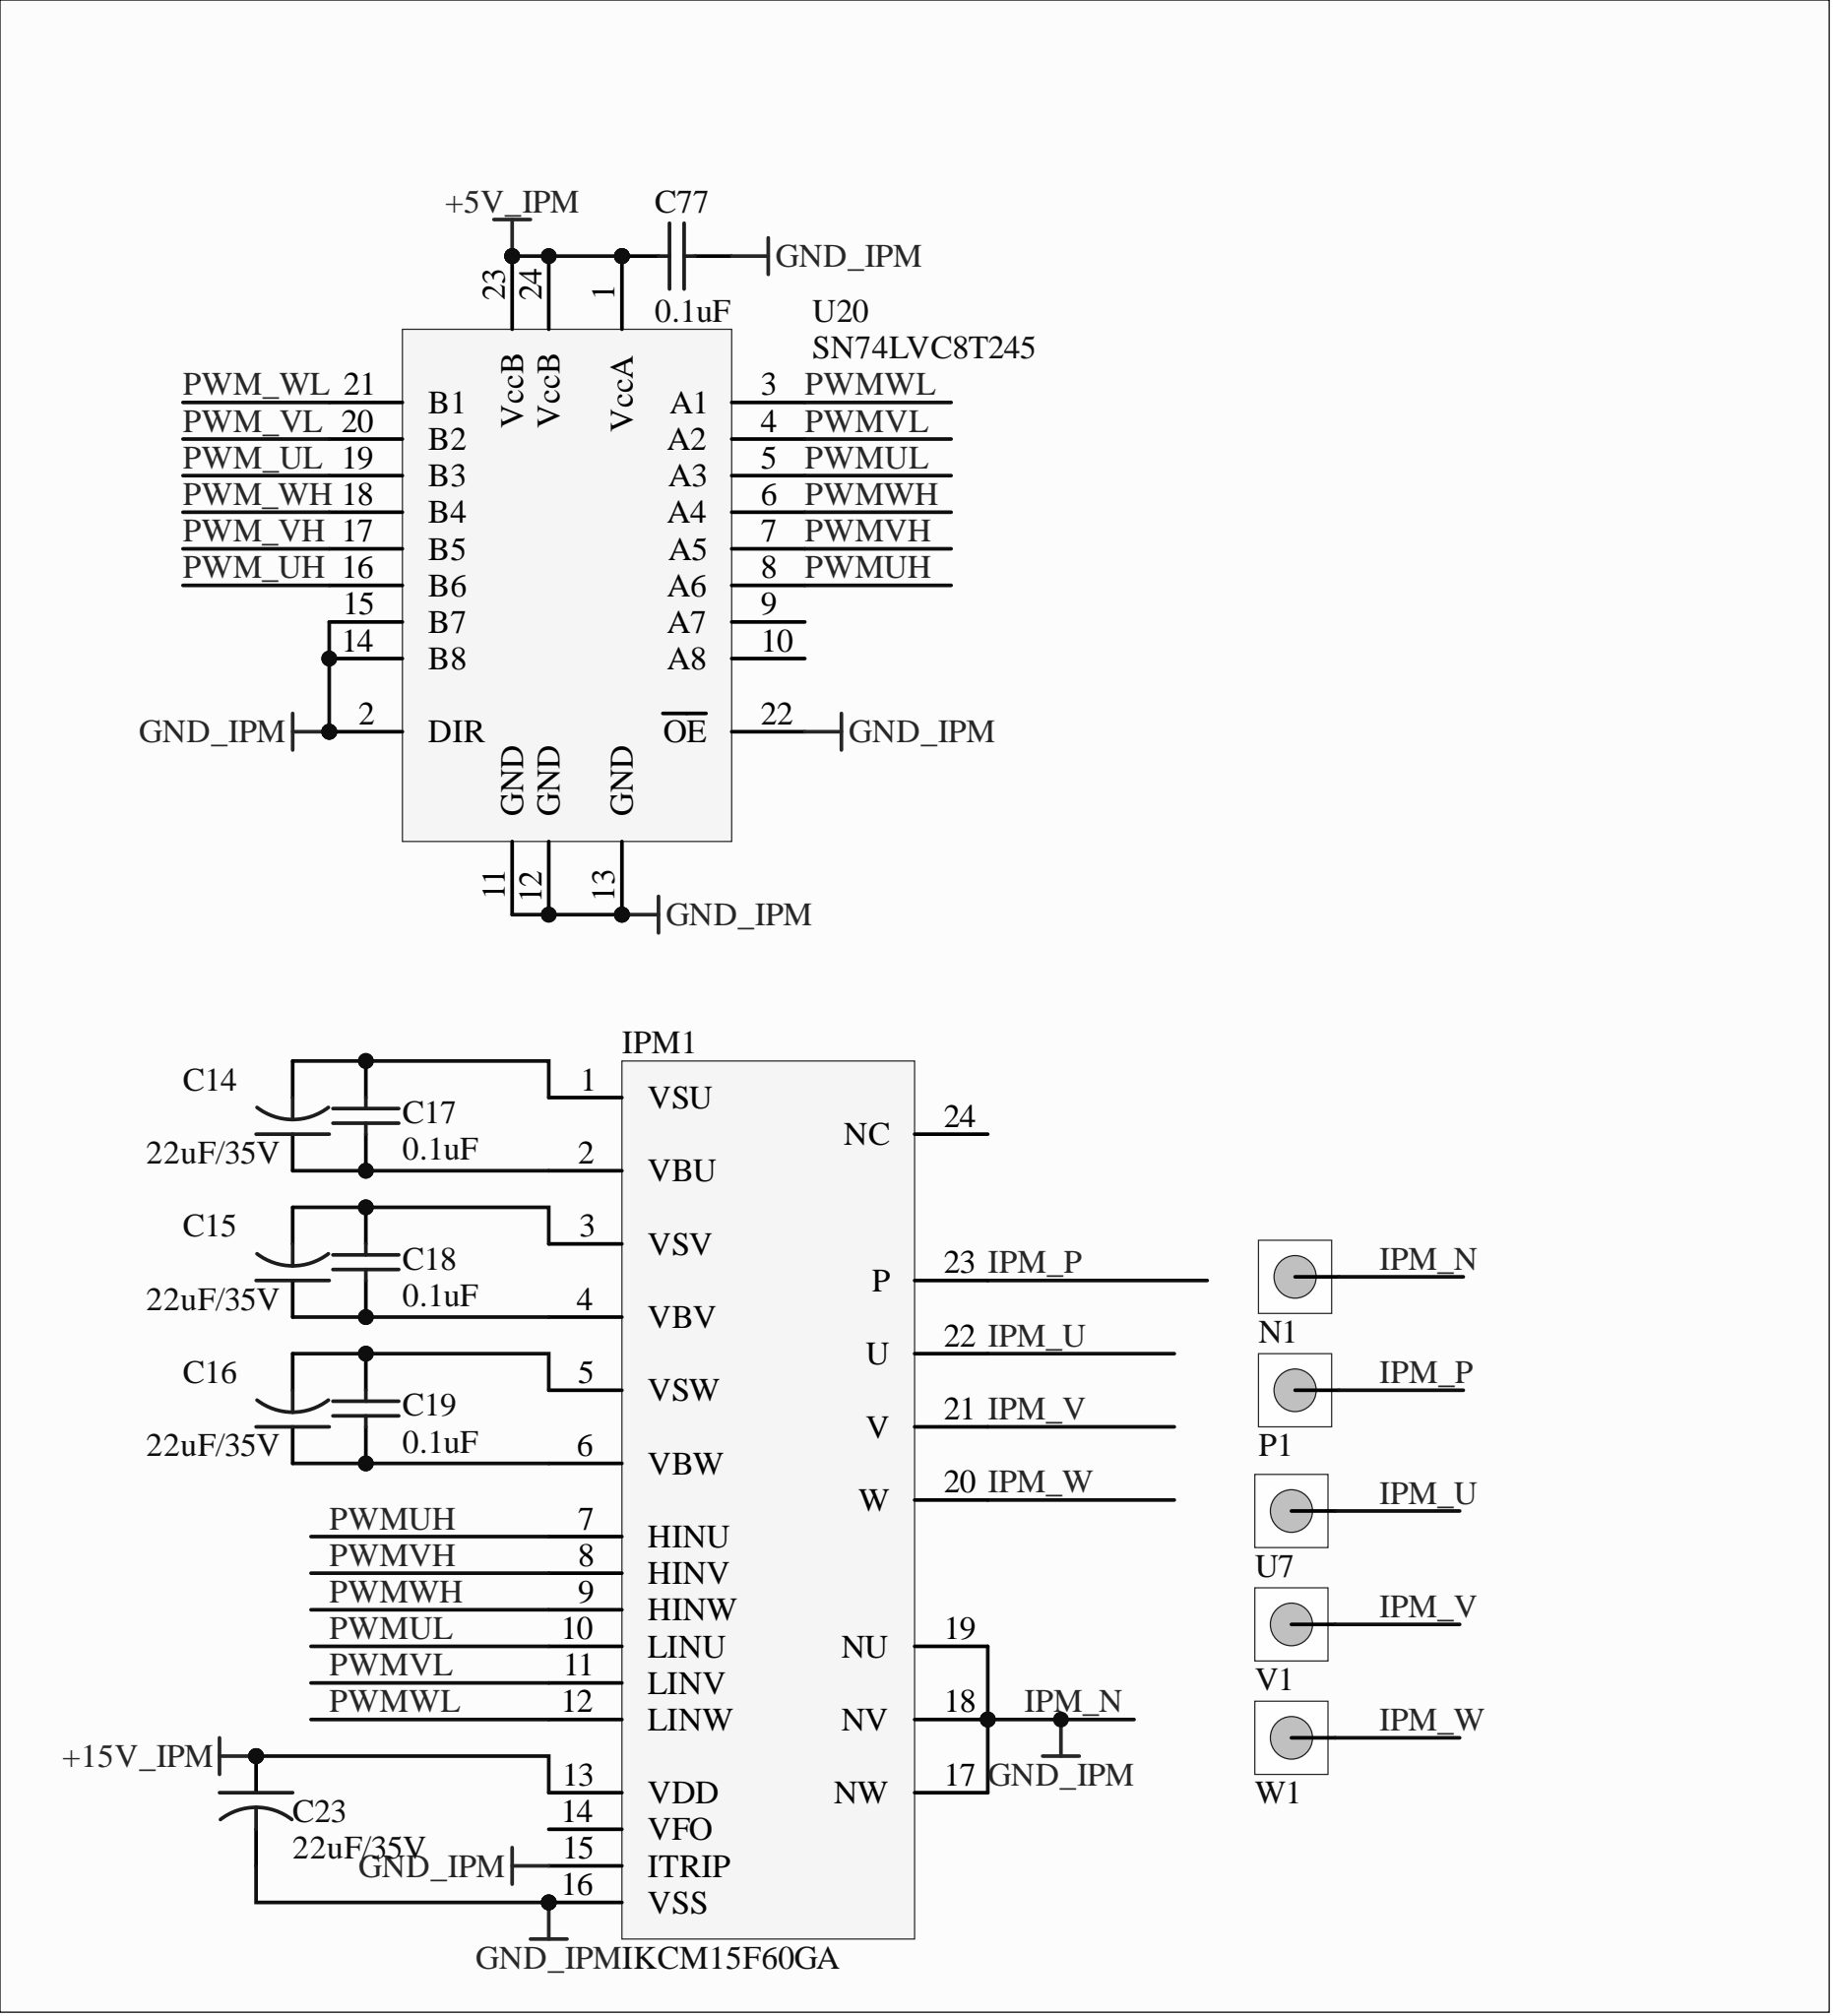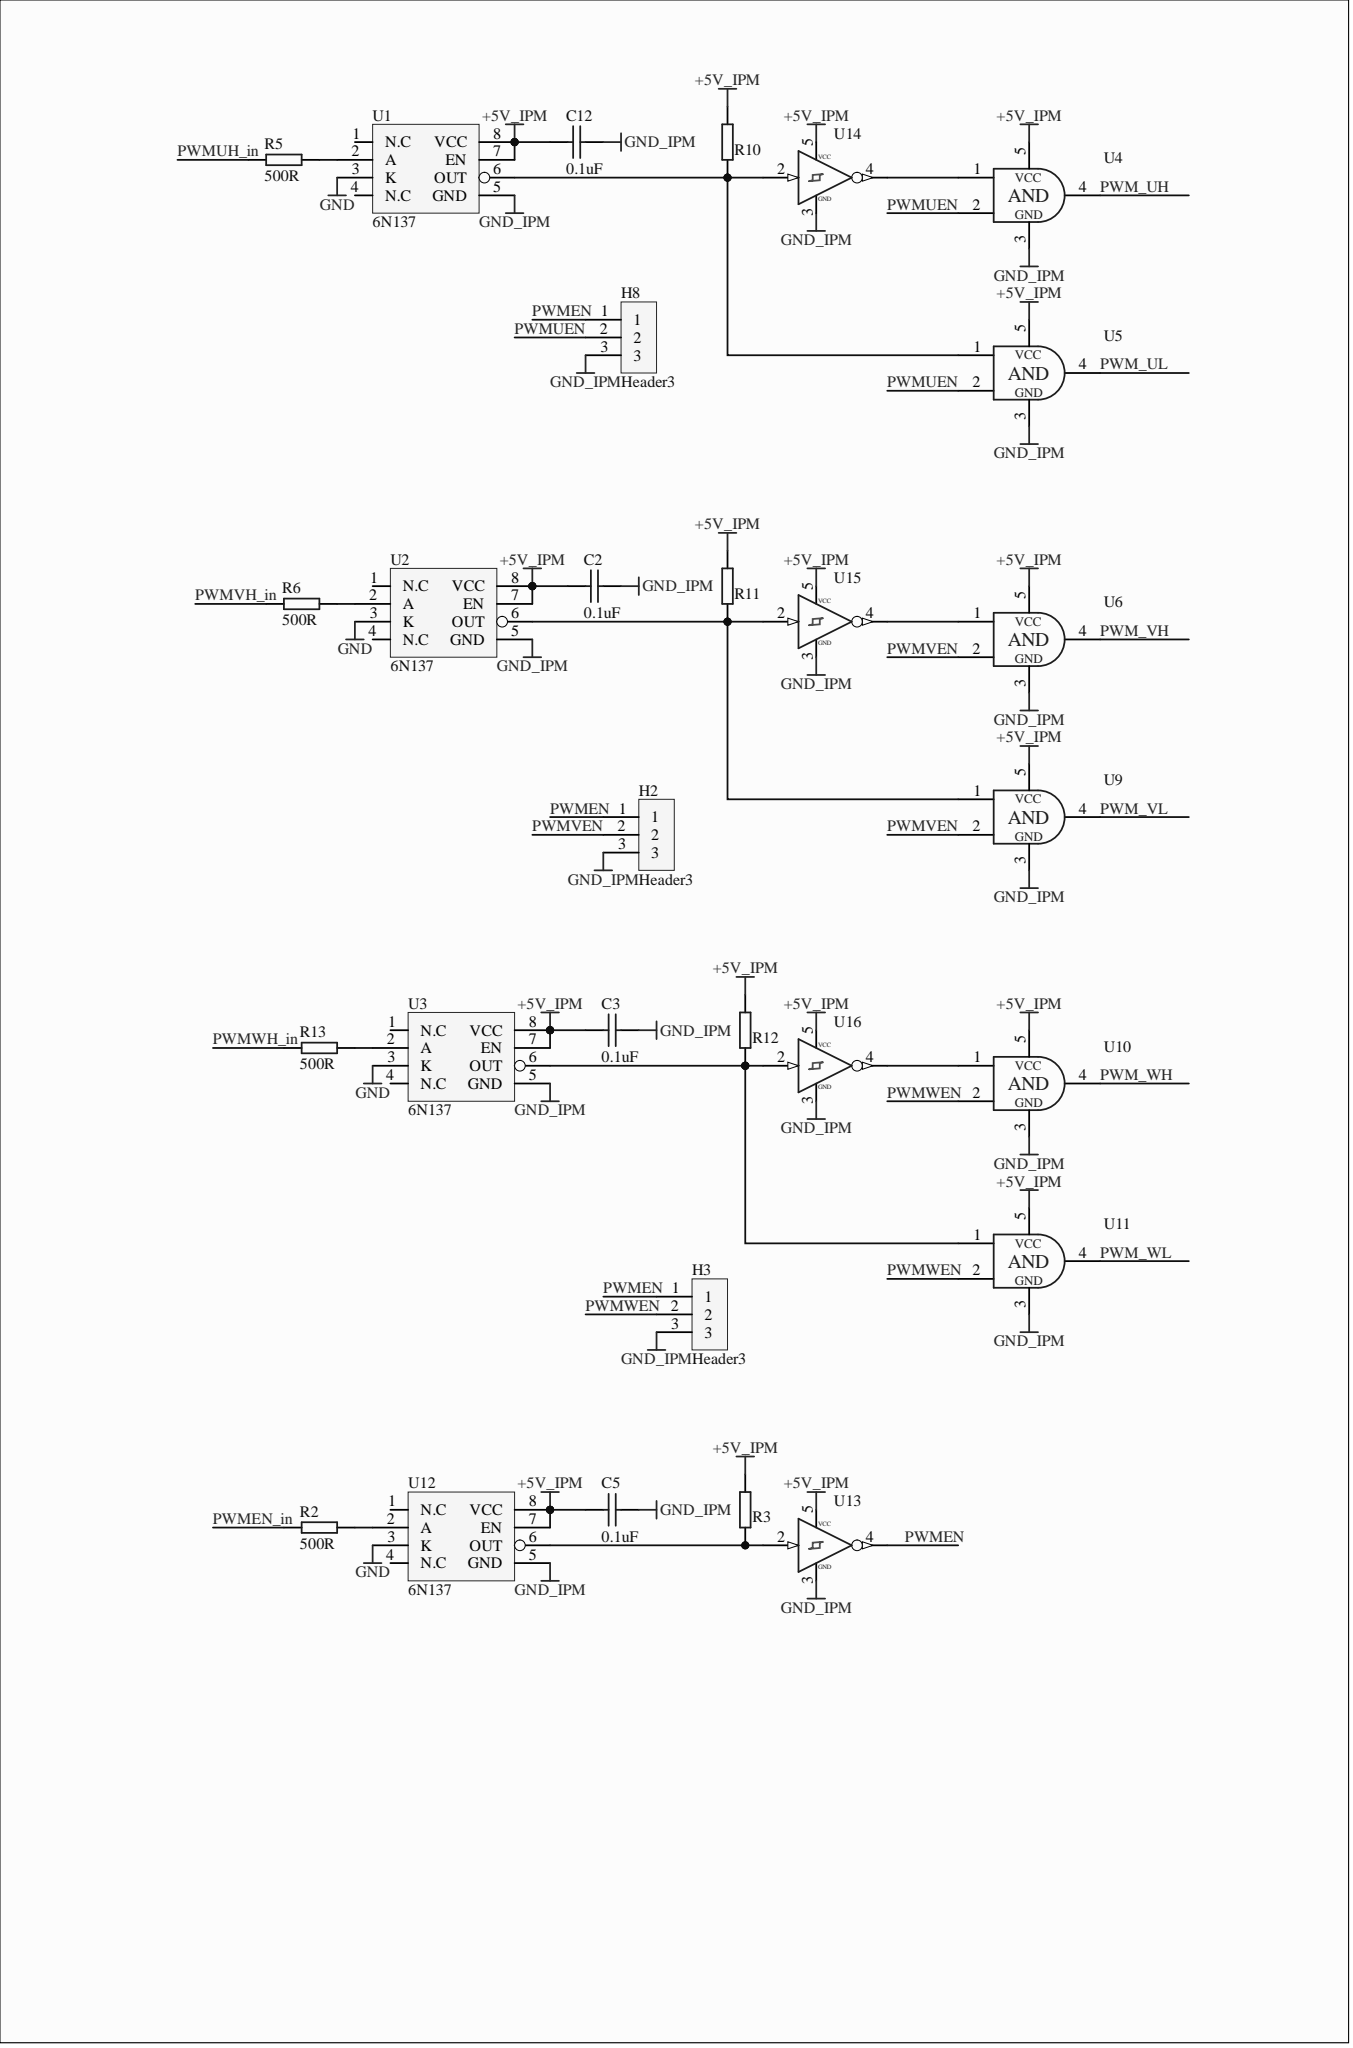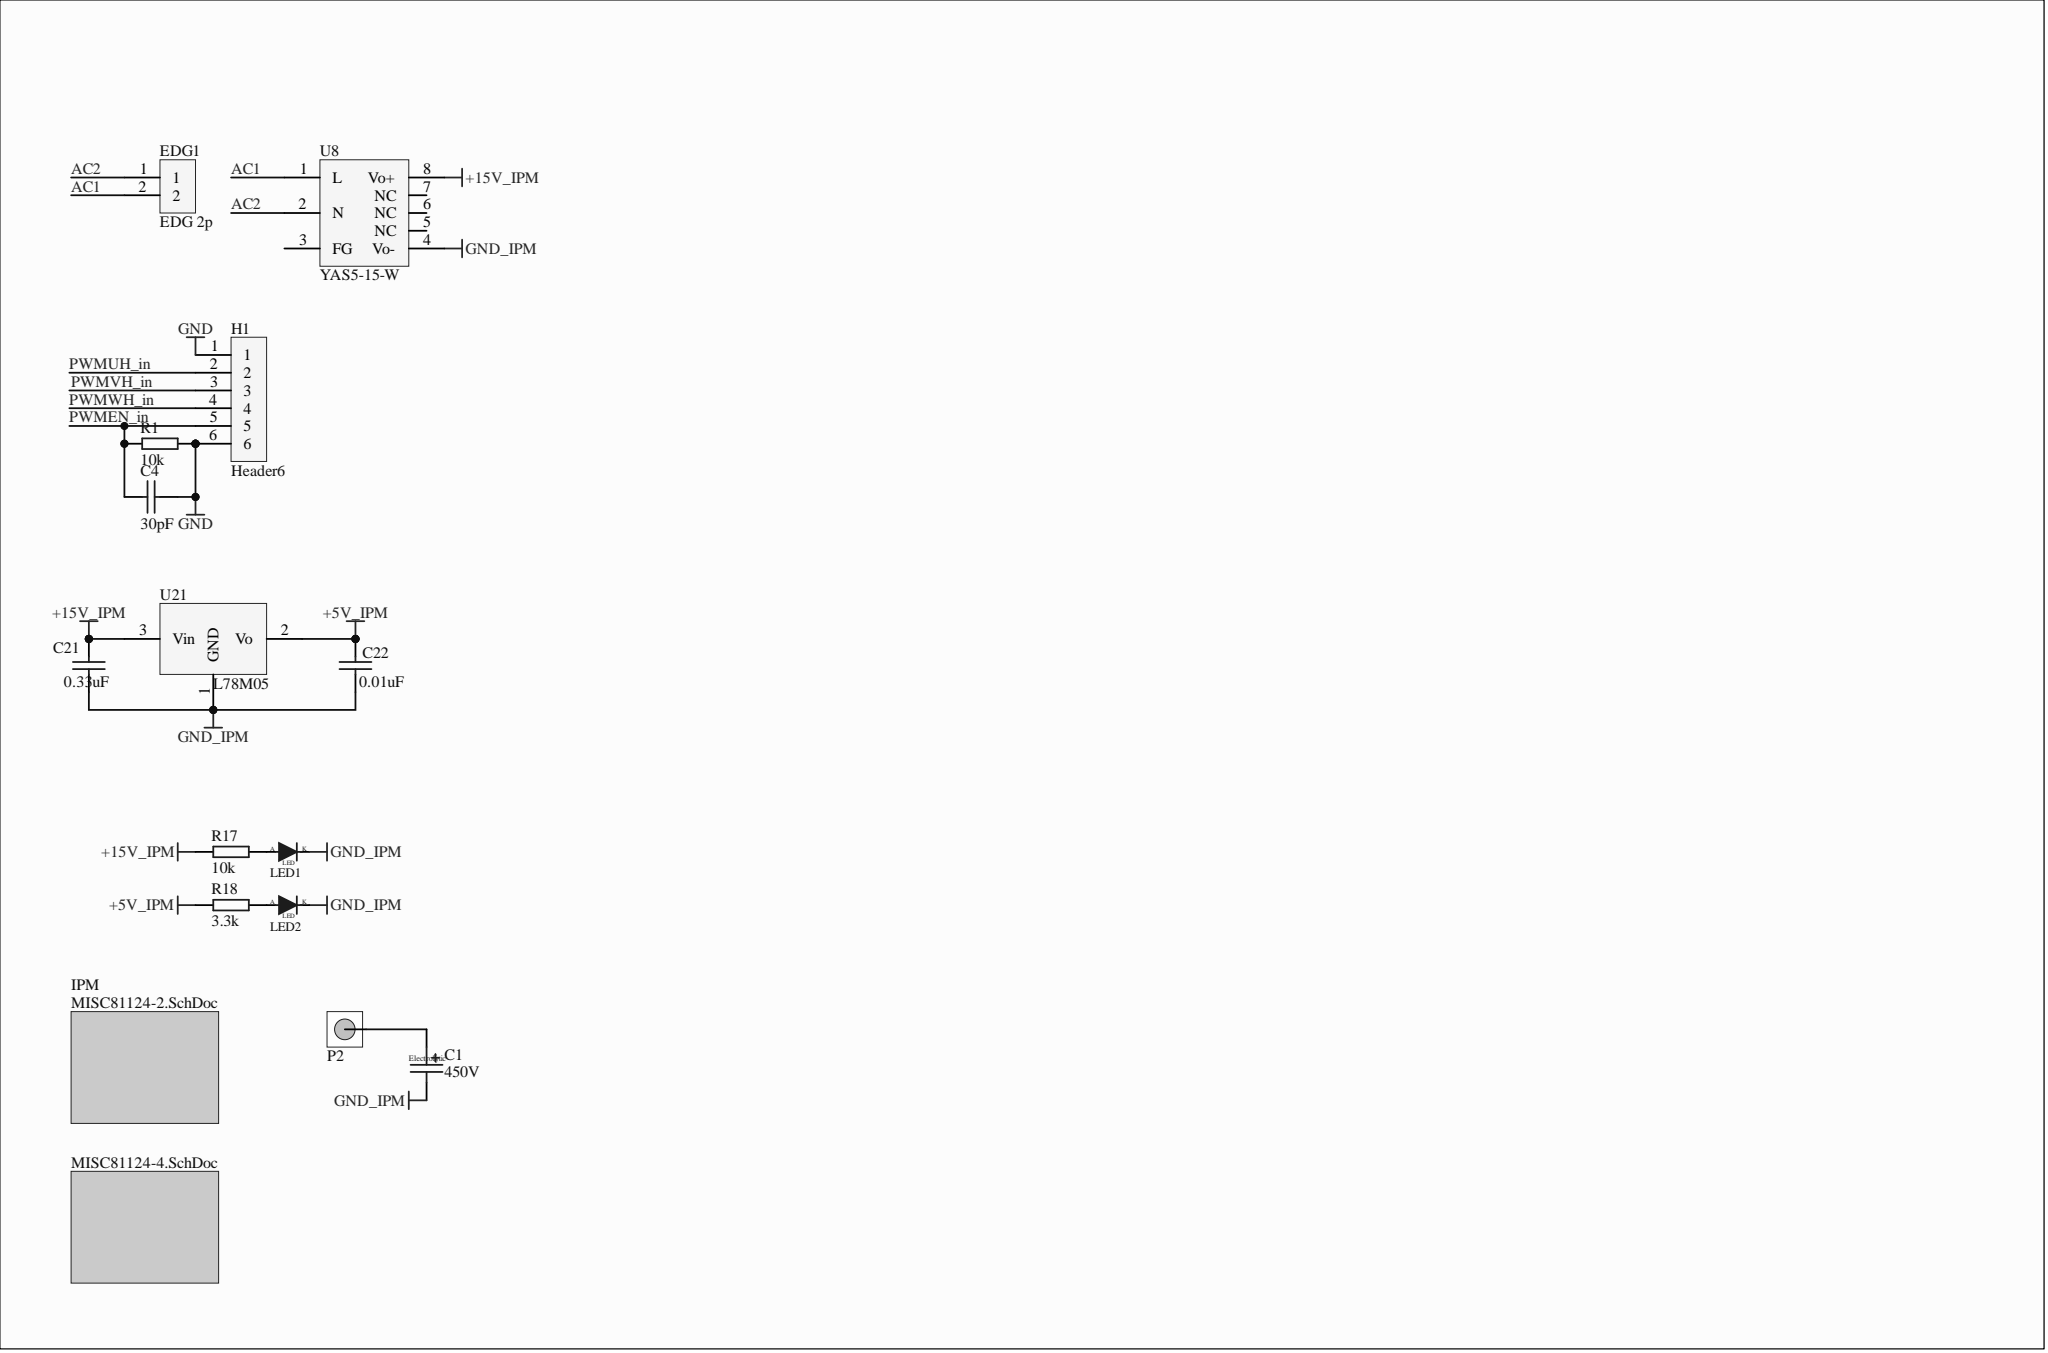Circuit board | Altium Designer | 58 parts | 50 nets
Bill of materials:
Comment,Description,Designator,Footprint,LibRef,Quantity
"450V","Electrolytic Capacitor(Pin1 Positive)","C1","ElecCap_450V","ELECTROCap","1"
"0.1uF","Capacitor","C2, C3, C5, C12, C17, C18, C19, C77","0805","CAP","8"
"30pF","Capacitor","C4","0805","CAP","1"
"22uF/35V","TaCap_D","C14, C15, C16, C23","7343_CASE-D","TaCap_D","4"
"0.33uF","Capacitor","C21","0805","CAP","1"
"0.01uF","Capacitor","C22","0805","CAP","1"
"EDG 2p","EDG 2p","EDG1","EDGCon_2p_3.81mm","EDG 2p","1"
"Header6","Header6","H1","EDGCon_6P_5.08mm","Header6","1"
"Header3","Header3","H2, H3, H8","PinHeader3_2.54mm","Header3","3"
"IKCM15F60GA","IKCM15F60GA","IPM1","IKCM15F60GA","IKCM15F60GA","1"
"LED","LED","LED1, LED2","0805_LED","LED","2"
"PCBTerminator","PCB terminal for high current","N1, P1, P2, U7, V1, W1","PCBTerminator","PCBTerminator","6"
"10k","","R1, R3, R10, R11, R12, R17","0805","RES2","6"
"500R","","R2, R5, R6, R13","1206","RES2","4"
"3.3k","","R18","0805","RES2","1"
"6N137","High-speed optocoupler","U1, U2, U3, U12","DIP-8","6N137","4"
"SN74AHC1G08","Single 2-Input Positive-AND Buffer","U4, U5, U6, U9, U10, U11","SOT-23-5","SN74AHC1G08","6"
"YAS5-15-W","YAS5-15-W","U8","YAS5","YAS5","1"
"SN74AHC1G04","Single Input Inverter","U13, U14, U15, U16","SOT-23-5","SN74AHC1G04","4"
"SN74LVC8T245","TI SN74LVC8T245PWR","U20","SN74LVC8T245_TSSOP24","SN74LVC8T245","1"
"L78M05","L78M05","U21","TO-252-2(DPAK)","LM1085ISX-3.3","1"
Netlist (Protel format):
[
C1
ElecCap_450V
450V



]
[
C2
0805
0.1uF



]
[
C3
0805
0.1uF



]
[
C4
0805
30pF



]
[
C5
0805
0.1uF



]
[
C12
0805
0.1uF



]
[
C14
7343_CASE-D
22uF/35V



]
[
C15
7343_CASE-D
22uF/35V



]
[
C16
7343_CASE-D
22uF/35V



]
[
C17
0805
0.1uF



]
[
C18
0805
0.1uF



]
[
C19
0805
0.1uF



]
[
C21
0805
0.33uF



]
[
C22
0805
0.01uF



]
[
C23
7343_CASE-D
22uF/35V



]
[
C77
0805
0.1uF



]
[
EDG1
EDGCon_2p_3.81mm
EDG 2p



]
[
H1
EDGCon_6P_5.08mm
Header6



]
[
H2
PinHeader3_2.54mm
Header3



]
[
H3
PinHeader3_2.54mm
Header3



]
[
H8
PinHeader3_2.54mm
Header3



]
[
IPM1
IKCM15F60GA
IKCM15F60GA



]
[
LED1
0805_LED
LED



]
[
LED2
0805_LED
LED



]
[
N1
PCBTerminator
PCBTerminator



]
[
P1
PCBTerminator
PCBTerminator



]
[
P2
PCBTerminator
PCBTerminator



]
[
R1
0805
10k



]
[
R2
1206
500R



]
[
R3
0805
10k



]
[
R5
1206
500R



]
[
R6
1206
500R



]
[
R10
0805
10k



]
[
R11
0805
10k



]
[
R12
0805
10k



]
[
R13
1206
500R



]
[
R17
0805
10k



]
[
R18
0805
3.3k



]
[
U1
DIP-8
6N137



]
[
U2
DIP-8
6N137



]
[
U3
DIP-8
6N137



]
[
U4
SOT-23-5
SN74AHC1G08



]
[
U5
SOT-23-5
SN74AHC1G08



]
[
U6
SOT-23-5
SN74AHC1G08



]
[
U7
PCBTerminator
PCBTerminator



]
[
U8
YAS5
YAS5-15-W



]
[
U9
SOT-23-5
SN74AHC1G08



]
[
U10
SOT-23-5
SN74AHC1G08



]
[
U11
SOT-23-5
SN74AHC1G08



]
[
U12
DIP-8
6N137



]
[
U13
SOT-23-5
SN74AHC1G04



]
[
U14
SOT-23-5
SN74AHC1G04



]
[
U15
SOT-23-5
SN74AHC1G04



]
[
U16
SOT-23-5
SN74AHC1G04



]
[
U20
SN74LVC8T245_TSSOP24
SN74LVC8T245



]
[
U21
TO-252-2(DPAK)
L78M05



]
[
V1
PCBTerminator
PCBTerminator



]
[
W1
PCBTerminator
PCBTerminator



]
(
PWMWL
IPM1-12
U20-3
)
(
PWMWH_in
H1-4
R13-2
)
(
PWMWH
IPM1-9
U20-6
)
(
PWMWEN
H3-2
U10-2
U11-2
)
(
PWMVL
IPM1-11
U20-4
)
(
PWMVH_in
H1-3
R6-2
)
(
PWMVH
IPM1-8
U20-7
)
(
PWMVEN
H2-2
U6-2
U9-2
)
(
PWMUL
IPM1-10
U20-5
)
(
PWMUH_in
H1-2
R5-2
)
(
PWMUH
IPM1-7
U20-8
)
(
PWMUEN
H8-2
U4-2
U5-2
)
(
PWMEN_in
C4-2
H1-5
R1-2
R2-2
)
(
PWMEN
H2-1
H3-1
H8-1
U13-4
)
(
PWM_WL
U11-4
U20-21
)
(
PWM_WH
U10-4
U20-18
)
(
PWM_VL
U9-4
U20-20
)
(
PWM_VH
U6-4
U20-17
)
(
PWM_UL
U5-4
U20-19
)
(
PWM_UH
U4-4
U20-16
)
(
NetU10_1
U10-1
U16-4
)
(
NetU6_1
U6-1
U15-4
)
(
NetU4_1
U4-1
U14-4
)
(
NetR13_1
R13-1
U3-2
)
(
NetR12_1
R12-1
U3-6
U11-1
U16-2
)
(
NetR11_1
R11-1
U2-6
U9-1
U15-2
)
(
NetR10_1
R10-1
U1-6
U5-1
U14-2
)
(
NetR6_1
R6-1
U2-2
)
(
NetR5_1
R5-1
U1-2
)
(
NetR3_1
R3-1
U12-6
U13-2
)
(
NetR2_1
R2-1
U12-2
)
(
NetLED2_A
LED2-A
R18-1
)
(
NetLED1_A
LED1-A
R17-1
)
(
NetC16_2
C16-2
C19-2
IPM1-5
)
(
NetC16_1
C16-1
C19-1
IPM1-6
)
(
NetC15_2
C15-2
C18-2
IPM1-3
)
(
NetC15_1
C15-1
C18-1
IPM1-4
)
(
NetC14_2
C14-2
C17-2
IPM1-1
)
(
NetC14_1
C14-1
C17-1
IPM1-2
)
(
NetC1_1
C1-1
P2-1
)
(
IPM_W
IPM1-20
W1-1
)
(
IPM_V
IPM1-21
V1-1
)
(
IPM_U
IPM1-22
U7-1
)
(
IPM_P
IPM1-23
P1-1
)
(
IPM_N
C1-2
C2-1
C3-1
C5-1
C12-1
C21-1
C22-1
C23-2
C77-2
H2-3
H3-3
H8-3
IPM1-15
IPM1-16
IPM1-17
IPM1-18
IPM1-19
LED1-K
LED2-K
N1-1
U1-5
U2-5
U3-5
U4-3
U5-3
U6-3
U8-4
U9-3
U10-3
U11-3
U12-5
U13-3
U14-3
U15-3
U16-3
U20-2
U20-11
U20-12
U20-13
U20-14
U20-15
U20-22
U21-1
)
(
GND
C4-1
H1-1
H1-6
R1-1
U1-3
U2-3
U3-3
U12-3
)
(
AC2
EDG1-1
U8-2
)
(
AC1
EDG1-2
U8-1
)
(
+15V_IPM
C21-2
C23-1
IPM1-13
R17-2
U8-8
U21-3
)
(
+5V_IPM
C2-2
C3-2
C5-2
C12-2
C22-2
C77-1
R3-2
R10-2
R11-2
R12-2
R18-2
U1-7
U1-8
U2-7
U2-8
U3-7
U3-8
U4-5
U5-5
U6-5
U9-5
U10-5
U11-5
U12-7
U12-8
U13-5
U14-5
U15-5
U16-5
U20-1
U20-23
U20-24
U21-2
)